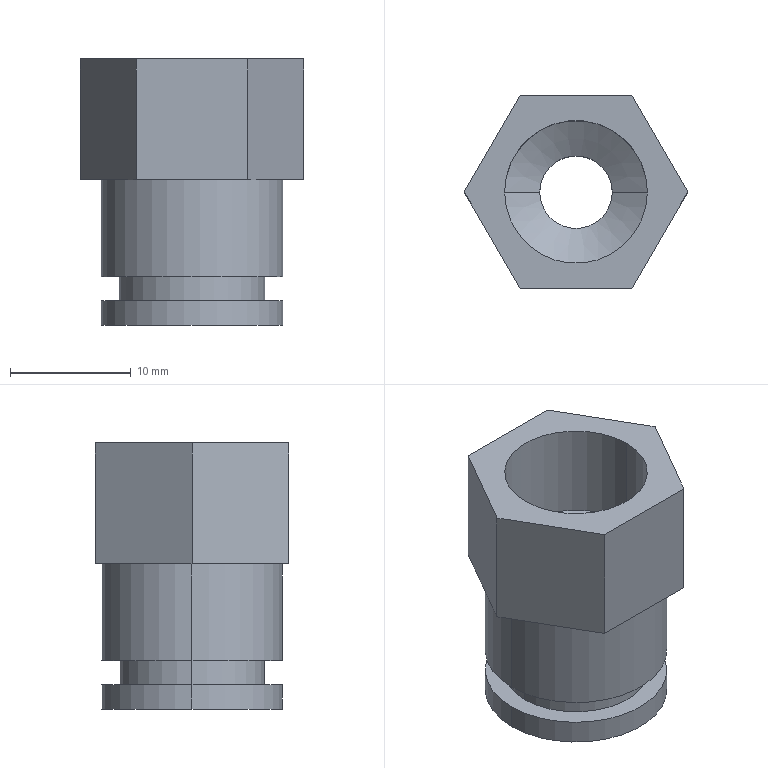Part | SolidWorks | features ICE 4, Extrusion 1, HoleWzd 1 | 1 solid | 23 faces | box 18.475 x 16 x 22 mm | volume 2877 mm3 | plane 11 | cylinder 10 | cone 2 | commonest cylinder face diameters 15 x4 6 x2 11.8 x2 12 x2
STEP:
#1=CARTESIAN_POINT('',(-5.9,0.,14.));
#2=VERTEX_POINT('',#1);
#3=CARTESIAN_POINT('',(5.9,0.,14.));
#4=VERTEX_POINT('',#3);
#5=CARTESIAN_POINT('',(0.,0.,14.));
#6=DIRECTION('',(0.,0.,1.));
#7=DIRECTION('',(1.,0.,0.));
#8=AXIS2_PLACEMENT_3D('',#5,#6,#7);
#9=CIRCLE('',#8,5.9);
#10=EDGE_CURVE('',#2,#4,#9,.T.);
#11=ORIENTED_EDGE('',*,*,#10,.F.);
#12=CARTESIAN_POINT('',(-5.9,0.,22.));
#13=VERTEX_POINT('',#12);
#14=CARTESIAN_POINT('',(-5.9,0.,22.));
#15=DIRECTION('',(0.,0.,1.));
#16=VECTOR('',#15,1000.);
#17=LINE('',#14,#16);
#18=EDGE_CURVE('',#2,#13,#17,.T.);
#19=ORIENTED_EDGE('',*,*,#18,.T.);
#20=CARTESIAN_POINT('',(5.9,0.,22.));
#21=VERTEX_POINT('',#20);
#22=CARTESIAN_POINT('',(0.,0.,22.));
#23=DIRECTION('',(0.,0.,1.));
#24=DIRECTION('',(1.,0.,0.));
#25=AXIS2_PLACEMENT_3D('',#22,#23,#24);
#26=CIRCLE('',#25,5.9);
#27=EDGE_CURVE('',#13,#21,#26,.T.);
#28=ORIENTED_EDGE('',*,*,#27,.T.);
#29=CARTESIAN_POINT('',(5.9,0.,22.));
#30=DIRECTION('',(0.,0.,1.));
#31=VECTOR('',#30,1000.);
#32=LINE('',#29,#31);
#33=EDGE_CURVE('',#4,#21,#32,.T.);
#34=ORIENTED_EDGE('',*,*,#33,.F.);
#35=EDGE_LOOP('',(#11,#19,#28,#34));
#36=FACE_OUTER_BOUND('',#35,.T.);
#37=CARTESIAN_POINT('',(0.,0.,22.));
#38=DIRECTION('',(0.,0.,1.));
#39=DIRECTION('',(1.,0.,0.));
#40=AXIS2_PLACEMENT_3D('',#37,#38,#39);
#41=CYLINDRICAL_SURFACE('',#40,5.9);
#42=ADVANCED_FACE('',(#36),#41,.F.);
#43=CARTESIAN_POINT('',(-3.,0.,12.258));
#44=VERTEX_POINT('',#43);
#45=CARTESIAN_POINT('',(3.,0.,12.258));
#46=VERTEX_POINT('',#45);
#47=CARTESIAN_POINT('',(0.,0.,12.258));
#48=DIRECTION('',(0.,0.,1.));
#49=DIRECTION('',(1.,0.,0.));
#50=AXIS2_PLACEMENT_3D('',#47,#48,#49);
#51=CIRCLE('',#50,3.);
#52=EDGE_CURVE('',#44,#46,#51,.T.);
#53=ORIENTED_EDGE('',*,*,#52,.F.);
#54=CARTESIAN_POINT('',(-5.9,0.,14.));
#55=DIRECTION('',(-0.8572,0.,0.515));
#56=VECTOR('',#55,1000.);
#57=LINE('',#54,#56);
#58=EDGE_CURVE('',#44,#2,#57,.T.);
#59=ORIENTED_EDGE('',*,*,#58,.T.);
#60=ORIENTED_EDGE('',*,*,#10,.T.);
#61=CARTESIAN_POINT('',(5.9,0.,14.));
#62=DIRECTION('',(0.8572,0.,0.515));
#63=VECTOR('',#62,1000.);
#64=LINE('',#61,#63);
#65=EDGE_CURVE('',#46,#4,#64,.T.);
#66=ORIENTED_EDGE('',*,*,#65,.F.);
#67=EDGE_LOOP('',(#53,#59,#60,#66));
#68=FACE_OUTER_BOUND('',#67,.T.);
#69=CARTESIAN_POINT('',(0.,0.,14.));
#70=DIRECTION('',(0.,0.,1.));
#71=DIRECTION('',(1.,0.,0.));
#72=AXIS2_PLACEMENT_3D('',#69,#70,#71);
#73=CONICAL_SURFACE('',#72,5.9,1.03);
#74=ADVANCED_FACE('',(#68),#73,.F.);
#75=ORIENTED_EDGE('',*,*,#52,.T.);
#76=CARTESIAN_POINT('',(3.,0.,0.));
#77=VERTEX_POINT('',#76);
#78=CARTESIAN_POINT('',(3.,0.,22.));
#79=DIRECTION('',(0.,0.,-1.));
#80=VECTOR('',#79,1000.);
#81=LINE('',#78,#80);
#82=EDGE_CURVE('',#46,#77,#81,.T.);
#83=ORIENTED_EDGE('',*,*,#82,.T.);
#84=CARTESIAN_POINT('',(-3.,0.,0.));
#85=VERTEX_POINT('',#84);
#86=CARTESIAN_POINT('',(0.,0.,0.));
#87=DIRECTION('',(0.,0.,-1.));
#88=DIRECTION('',(-1.,0.,0.));
#89=AXIS2_PLACEMENT_3D('',#86,#87,#88);
#90=CIRCLE('',#89,3.);
#91=EDGE_CURVE('',#77,#85,#90,.T.);
#92=ORIENTED_EDGE('',*,*,#91,.T.);
#93=CARTESIAN_POINT('',(-3.,0.,22.));
#94=DIRECTION('',(0.,0.,-1.));
#95=VECTOR('',#94,1000.);
#96=LINE('',#93,#95);
#97=EDGE_CURVE('',#44,#85,#96,.T.);
#98=ORIENTED_EDGE('',*,*,#97,.F.);
#99=EDGE_LOOP('',(#75,#83,#92,#98));
#100=FACE_OUTER_BOUND('',#99,.T.);
#101=CARTESIAN_POINT('',(0.,0.,22.));
#102=DIRECTION('',(0.,0.,-1.));
#103=DIRECTION('',(-1.,0.,0.));
#104=AXIS2_PLACEMENT_3D('',#101,#102,#103);
#105=CYLINDRICAL_SURFACE('',#104,3.);
#106=ADVANCED_FACE('',(#100),#105,.F.);
#107=CARTESIAN_POINT('',(7.5,0.,12.));
#108=VERTEX_POINT('',#107);
#109=CARTESIAN_POINT('',(-7.5,0.,12.));
#110=VERTEX_POINT('',#109);
#111=CARTESIAN_POINT('',(0.,0.,12.));
#112=DIRECTION('',(0.,0.,1.));
#113=DIRECTION('',(1.,0.,0.));
#114=AXIS2_PLACEMENT_3D('',#111,#112,#113);
#115=CIRCLE('',#114,7.5);
#116=EDGE_CURVE('',#108,#110,#115,.T.);
#117=ORIENTED_EDGE('',*,*,#116,.F.);
#118=CARTESIAN_POINT('',(7.5,0.,4.));
#119=VERTEX_POINT('',#118);
#120=CARTESIAN_POINT('',(7.5,0.,12.));
#121=DIRECTION('',(0.,0.,-1.));
#122=VECTOR('',#121,1000.);
#123=LINE('',#120,#122);
#124=EDGE_CURVE('',#108,#119,#123,.T.);
#125=ORIENTED_EDGE('',*,*,#124,.T.);
#126=CARTESIAN_POINT('',(-7.5,0.,4.));
#127=VERTEX_POINT('',#126);
#128=CARTESIAN_POINT('',(0.,0.,4.));
#129=DIRECTION('',(0.,0.,1.));
#130=DIRECTION('',(1.,0.,0.));
#131=AXIS2_PLACEMENT_3D('',#128,#129,#130);
#132=CIRCLE('',#131,7.5);
#133=EDGE_CURVE('',#119,#127,#132,.T.);
#134=ORIENTED_EDGE('',*,*,#133,.T.);
#135=CARTESIAN_POINT('',(-7.5,0.,12.));
#136=DIRECTION('',(0.,0.,-1.));
#137=VECTOR('',#136,1000.);
#138=LINE('',#135,#137);
#139=EDGE_CURVE('',#110,#127,#138,.T.);
#140=ORIENTED_EDGE('',*,*,#139,.F.);
#141=EDGE_LOOP('',(#117,#125,#134,#140));
#142=FACE_OUTER_BOUND('',#141,.T.);
#143=CARTESIAN_POINT('',(0.,0.,12.));
#144=DIRECTION('',(0.,0.,-1.));
#145=DIRECTION('',(-1.,0.,0.));
#146=AXIS2_PLACEMENT_3D('',#143,#144,#145);
#147=CYLINDRICAL_SURFACE('',#146,7.5);
#148=ADVANCED_FACE('',(#142),#147,.T.);
#149=CARTESIAN_POINT('',(6.,0.,4.));
#150=VERTEX_POINT('',#149);
#151=CARTESIAN_POINT('',(-6.,0.,4.));
#152=VERTEX_POINT('',#151);
#153=CARTESIAN_POINT('',(0.,0.,4.));
#154=DIRECTION('',(0.,0.,1.));
#155=DIRECTION('',(1.,0.,0.));
#156=AXIS2_PLACEMENT_3D('',#153,#154,#155);
#157=CIRCLE('',#156,6.);
#158=EDGE_CURVE('',#150,#152,#157,.T.);
#159=ORIENTED_EDGE('',*,*,#158,.F.);
#160=CARTESIAN_POINT('',(6.,0.,2.));
#161=VERTEX_POINT('',#160);
#162=CARTESIAN_POINT('',(6.,0.,4.));
#163=DIRECTION('',(0.,0.,-1.));
#164=VECTOR('',#163,1000.);
#165=LINE('',#162,#164);
#166=EDGE_CURVE('',#150,#161,#165,.T.);
#167=ORIENTED_EDGE('',*,*,#166,.T.);
#168=CARTESIAN_POINT('',(-6.,0.,2.));
#169=VERTEX_POINT('',#168);
#170=CARTESIAN_POINT('',(0.,0.,2.));
#171=DIRECTION('',(0.,0.,1.));
#172=DIRECTION('',(1.,0.,0.));
#173=AXIS2_PLACEMENT_3D('',#170,#171,#172);
#174=CIRCLE('',#173,6.);
#175=EDGE_CURVE('',#161,#169,#174,.T.);
#176=ORIENTED_EDGE('',*,*,#175,.T.);
#177=CARTESIAN_POINT('',(-6.,0.,4.));
#178=DIRECTION('',(0.,0.,-1.));
#179=VECTOR('',#178,1000.);
#180=LINE('',#177,#179);
#181=EDGE_CURVE('',#152,#169,#180,.T.);
#182=ORIENTED_EDGE('',*,*,#181,.F.);
#183=EDGE_LOOP('',(#159,#167,#176,#182));
#184=FACE_OUTER_BOUND('',#183,.T.);
#185=CARTESIAN_POINT('',(0.,0.,4.));
#186=DIRECTION('',(0.,0.,-1.));
#187=DIRECTION('',(-1.,0.,0.));
#188=AXIS2_PLACEMENT_3D('',#185,#186,#187);
#189=CYLINDRICAL_SURFACE('',#188,6.);
#190=ADVANCED_FACE('',(#184),#189,.T.);
#191=CARTESIAN_POINT('',(7.5,0.,2.));
#192=VERTEX_POINT('',#191);
#193=CARTESIAN_POINT('',(-7.5,0.,2.));
#194=VERTEX_POINT('',#193);
#195=CARTESIAN_POINT('',(0.,0.,2.));
#196=DIRECTION('',(0.,0.,1.));
#197=DIRECTION('',(1.,0.,0.));
#198=AXIS2_PLACEMENT_3D('',#195,#196,#197);
#199=CIRCLE('',#198,7.5);
#200=EDGE_CURVE('',#192,#194,#199,.T.);
#201=ORIENTED_EDGE('',*,*,#200,.F.);
#202=CARTESIAN_POINT('',(7.5,0.,0.));
#203=VERTEX_POINT('',#202);
#204=CARTESIAN_POINT('',(7.5,0.,2.));
#205=DIRECTION('',(0.,0.,-1.));
#206=VECTOR('',#205,1000.);
#207=LINE('',#204,#206);
#208=EDGE_CURVE('',#192,#203,#207,.T.);
#209=ORIENTED_EDGE('',*,*,#208,.T.);
#210=CARTESIAN_POINT('',(-7.5,0.,0.));
#211=VERTEX_POINT('',#210);
#212=CARTESIAN_POINT('',(0.,0.,0.));
#213=DIRECTION('',(0.,0.,1.));
#214=DIRECTION('',(1.,0.,0.));
#215=AXIS2_PLACEMENT_3D('',#212,#213,#214);
#216=CIRCLE('',#215,7.5);
#217=EDGE_CURVE('',#203,#211,#216,.T.);
#218=ORIENTED_EDGE('',*,*,#217,.T.);
#219=CARTESIAN_POINT('',(-7.5,0.,2.));
#220=DIRECTION('',(0.,0.,-1.));
#221=VECTOR('',#220,1000.);
#222=LINE('',#219,#221);
#223=EDGE_CURVE('',#194,#211,#222,.T.);
#224=ORIENTED_EDGE('',*,*,#223,.F.);
#225=EDGE_LOOP('',(#201,#209,#218,#224));
#226=FACE_OUTER_BOUND('',#225,.T.);
#227=CARTESIAN_POINT('',(0.,0.,2.));
#228=DIRECTION('',(0.,0.,-1.));
#229=DIRECTION('',(-1.,0.,0.));
#230=AXIS2_PLACEMENT_3D('',#227,#228,#229);
#231=CYLINDRICAL_SURFACE('',#230,7.5);
#232=ADVANCED_FACE('',(#226),#231,.T.);
#233=ORIENTED_EDGE('',*,*,#208,.F.);
#234=CARTESIAN_POINT('',(0.,0.,2.));
#235=DIRECTION('',(0.,0.,1.));
#236=DIRECTION('',(1.,0.,0.));
#237=AXIS2_PLACEMENT_3D('',#234,#235,#236);
#238=CIRCLE('',#237,7.5);
#239=EDGE_CURVE('',#194,#192,#238,.T.);
#240=ORIENTED_EDGE('',*,*,#239,.F.);
#241=ORIENTED_EDGE('',*,*,#223,.T.);
#242=CARTESIAN_POINT('',(0.,0.,0.));
#243=DIRECTION('',(0.,0.,1.));
#244=DIRECTION('',(1.,0.,0.));
#245=AXIS2_PLACEMENT_3D('',#242,#243,#244);
#246=CIRCLE('',#245,7.5);
#247=EDGE_CURVE('',#211,#203,#246,.T.);
#248=ORIENTED_EDGE('',*,*,#247,.T.);
#249=EDGE_LOOP('',(#233,#240,#241,#248));
#250=FACE_OUTER_BOUND('',#249,.T.);
#251=CARTESIAN_POINT('',(0.,0.,2.));
#252=DIRECTION('',(0.,0.,-1.));
#253=DIRECTION('',(-1.,0.,0.));
#254=AXIS2_PLACEMENT_3D('',#251,#252,#253);
#255=CYLINDRICAL_SURFACE('',#254,7.5);
#256=ADVANCED_FACE('',(#250),#255,.T.);
#257=CARTESIAN_POINT('',(0.,0.,2.));
#258=DIRECTION('',(0.,0.,1.));
#259=DIRECTION('',(1.,0.,0.));
#260=AXIS2_PLACEMENT_3D('',#257,#258,#259);
#261=CIRCLE('',#260,6.);
#262=EDGE_CURVE('',#169,#161,#261,.T.);
#263=ORIENTED_EDGE('',*,*,#262,.F.);
#264=ORIENTED_EDGE('',*,*,#175,.F.);
#265=EDGE_LOOP('',(#263,#264));
#266=FACE_BOUND('',#265,.T.);
#267=ORIENTED_EDGE('',*,*,#239,.T.);
#268=ORIENTED_EDGE('',*,*,#200,.T.);
#269=EDGE_LOOP('',(#267,#268));
#270=FACE_OUTER_BOUND('',#269,.T.);
#271=CARTESIAN_POINT('',(0.,0.,2.));
#272=DIRECTION('',(0.,0.,1.));
#273=DIRECTION('',(1.,0.,0.));
#274=AXIS2_PLACEMENT_3D('',#271,#272,#273);
#275=PLANE('',#274);
#276=ADVANCED_FACE('',(#266,#270),#275,.T.);
#277=CARTESIAN_POINT('',(0.,0.,0.));
#278=DIRECTION('',(0.,0.,-1.));
#279=DIRECTION('',(-1.,0.,0.));
#280=AXIS2_PLACEMENT_3D('',#277,#278,#279);
#281=CIRCLE('',#280,3.);
#282=EDGE_CURVE('',#85,#77,#281,.T.);
#283=ORIENTED_EDGE('',*,*,#282,.F.);
#284=ORIENTED_EDGE('',*,*,#91,.F.);
#285=EDGE_LOOP('',(#283,#284));
#286=FACE_BOUND('',#285,.T.);
#287=ORIENTED_EDGE('',*,*,#247,.F.);
#288=ORIENTED_EDGE('',*,*,#217,.F.);
#289=EDGE_LOOP('',(#287,#288));
#290=FACE_OUTER_BOUND('',#289,.T.);
#291=CARTESIAN_POINT('',(0.,0.,0.));
#292=DIRECTION('',(0.,0.,1.));
#293=DIRECTION('',(1.,0.,0.));
#294=AXIS2_PLACEMENT_3D('',#291,#292,#293);
#295=PLANE('',#294);
#296=ADVANCED_FACE('',(#286,#290),#295,.F.);
#297=ORIENTED_EDGE('',*,*,#166,.F.);
#298=CARTESIAN_POINT('',(0.,0.,4.));
#299=DIRECTION('',(0.,0.,1.));
#300=DIRECTION('',(1.,0.,0.));
#301=AXIS2_PLACEMENT_3D('',#298,#299,#300);
#302=CIRCLE('',#301,6.);
#303=EDGE_CURVE('',#152,#150,#302,.T.);
#304=ORIENTED_EDGE('',*,*,#303,.F.);
#305=ORIENTED_EDGE('',*,*,#181,.T.);
#306=ORIENTED_EDGE('',*,*,#262,.T.);
#307=EDGE_LOOP('',(#297,#304,#305,#306));
#308=FACE_OUTER_BOUND('',#307,.T.);
#309=CARTESIAN_POINT('',(0.,0.,4.));
#310=DIRECTION('',(0.,0.,-1.));
#311=DIRECTION('',(-1.,0.,0.));
#312=AXIS2_PLACEMENT_3D('',#309,#310,#311);
#313=CYLINDRICAL_SURFACE('',#312,6.);
#314=ADVANCED_FACE('',(#308),#313,.T.);
#315=ORIENTED_EDGE('',*,*,#124,.F.);
#316=CARTESIAN_POINT('',(0.,0.,12.));
#317=DIRECTION('',(0.,0.,1.));
#318=DIRECTION('',(1.,0.,0.));
#319=AXIS2_PLACEMENT_3D('',#316,#317,#318);
#320=CIRCLE('',#319,7.5);
#321=EDGE_CURVE('',#110,#108,#320,.T.);
#322=ORIENTED_EDGE('',*,*,#321,.F.);
#323=ORIENTED_EDGE('',*,*,#139,.T.);
#324=CARTESIAN_POINT('',(0.,0.,4.));
#325=DIRECTION('',(0.,0.,1.));
#326=DIRECTION('',(1.,0.,0.));
#327=AXIS2_PLACEMENT_3D('',#324,#325,#326);
#328=CIRCLE('',#327,7.5);
#329=EDGE_CURVE('',#127,#119,#328,.T.);
#330=ORIENTED_EDGE('',*,*,#329,.T.);
#331=EDGE_LOOP('',(#315,#322,#323,#330));
#332=FACE_OUTER_BOUND('',#331,.T.);
#333=CARTESIAN_POINT('',(0.,0.,12.));
#334=DIRECTION('',(0.,0.,-1.));
#335=DIRECTION('',(-1.,0.,0.));
#336=AXIS2_PLACEMENT_3D('',#333,#334,#335);
#337=CYLINDRICAL_SURFACE('',#336,7.5);
#338=ADVANCED_FACE('',(#332),#337,.T.);
#339=ORIENTED_EDGE('',*,*,#303,.T.);
#340=ORIENTED_EDGE('',*,*,#158,.T.);
#341=EDGE_LOOP('',(#339,#340));
#342=FACE_BOUND('',#341,.T.);
#343=ORIENTED_EDGE('',*,*,#329,.F.);
#344=ORIENTED_EDGE('',*,*,#133,.F.);
#345=EDGE_LOOP('',(#343,#344));
#346=FACE_OUTER_BOUND('',#345,.T.);
#347=CARTESIAN_POINT('',(0.,0.,4.));
#348=DIRECTION('',(0.,0.,1.));
#349=DIRECTION('',(1.,0.,0.));
#350=AXIS2_PLACEMENT_3D('',#347,#348,#349);
#351=PLANE('',#350);
#352=ADVANCED_FACE('',(#342,#346),#351,.F.);
#353=CARTESIAN_POINT('',(4.619,-8.,12.));
#354=VERTEX_POINT('',#353);
#355=CARTESIAN_POINT('',(9.238,0.,12.));
#356=VERTEX_POINT('',#355);
#357=CARTESIAN_POINT('',(4.619,-8.,12.));
#358=DIRECTION('',(0.5,0.866,0.));
#359=VECTOR('',#358,1000.);
#360=LINE('',#357,#359);
#361=EDGE_CURVE('',#354,#356,#360,.T.);
#362=ORIENTED_EDGE('',*,*,#361,.T.);
#363=CARTESIAN_POINT('',(9.238,0.,22.));
#364=VERTEX_POINT('',#363);
#365=CARTESIAN_POINT('',(9.238,0.,22.));
#366=DIRECTION('',(0.,0.,-1.));
#367=VECTOR('',#366,1000.);
#368=LINE('',#365,#367);
#369=EDGE_CURVE('',#364,#356,#368,.T.);
#370=ORIENTED_EDGE('',*,*,#369,.F.);
#371=CARTESIAN_POINT('',(4.619,-8.,22.));
#372=VERTEX_POINT('',#371);
#373=CARTESIAN_POINT('',(4.619,-8.,22.));
#374=DIRECTION('',(0.5,0.866,0.));
#375=VECTOR('',#374,1000.);
#376=LINE('',#373,#375);
#377=EDGE_CURVE('',#372,#364,#376,.T.);
#378=ORIENTED_EDGE('',*,*,#377,.F.);
#379=CARTESIAN_POINT('',(4.619,-8.,22.));
#380=DIRECTION('',(0.,0.,-1.));
#381=VECTOR('',#380,1000.);
#382=LINE('',#379,#381);
#383=EDGE_CURVE('',#372,#354,#382,.T.);
#384=ORIENTED_EDGE('',*,*,#383,.T.);
#385=EDGE_LOOP('',(#362,#370,#378,#384));
#386=FACE_OUTER_BOUND('',#385,.T.);
#387=CARTESIAN_POINT('',(4.619,-8.,22.));
#388=DIRECTION('',(-0.866,0.5,0.));
#389=DIRECTION('',(-0.5,-0.866,0.));
#390=AXIS2_PLACEMENT_3D('',#387,#388,#389);
#391=PLANE('',#390);
#392=ADVANCED_FACE('',(#386),#391,.F.);
#393=CARTESIAN_POINT('',(4.619,8.,12.));
#394=VERTEX_POINT('',#393);
#395=CARTESIAN_POINT('',(9.238,0.,12.));
#396=DIRECTION('',(-0.5,0.866,0.));
#397=VECTOR('',#396,1000.);
#398=LINE('',#395,#397);
#399=EDGE_CURVE('',#356,#394,#398,.T.);
#400=ORIENTED_EDGE('',*,*,#399,.T.);
#401=CARTESIAN_POINT('',(4.619,8.,22.));
#402=VERTEX_POINT('',#401);
#403=CARTESIAN_POINT('',(4.619,8.,22.));
#404=DIRECTION('',(0.,0.,-1.));
#405=VECTOR('',#404,1000.);
#406=LINE('',#403,#405);
#407=EDGE_CURVE('',#402,#394,#406,.T.);
#408=ORIENTED_EDGE('',*,*,#407,.F.);
#409=CARTESIAN_POINT('',(9.238,0.,22.));
#410=DIRECTION('',(-0.5,0.866,0.));
#411=VECTOR('',#410,1000.);
#412=LINE('',#409,#411);
#413=EDGE_CURVE('',#364,#402,#412,.T.);
#414=ORIENTED_EDGE('',*,*,#413,.F.);
#415=ORIENTED_EDGE('',*,*,#369,.T.);
#416=EDGE_LOOP('',(#400,#408,#414,#415));
#417=FACE_OUTER_BOUND('',#416,.T.);
#418=CARTESIAN_POINT('',(9.238,0.,22.));
#419=DIRECTION('',(-0.866,-0.5,0.));
#420=DIRECTION('',(0.5,-0.866,0.));
#421=AXIS2_PLACEMENT_3D('',#418,#419,#420);
#422=PLANE('',#421);
#423=ADVANCED_FACE('',(#417),#422,.F.);
#424=CARTESIAN_POINT('',(-4.619,8.,12.));
#425=VERTEX_POINT('',#424);
#426=CARTESIAN_POINT('',(4.619,8.,12.));
#427=DIRECTION('',(-1.,0.,0.));
#428=VECTOR('',#427,1000.);
#429=LINE('',#426,#428);
#430=EDGE_CURVE('',#394,#425,#429,.T.);
#431=ORIENTED_EDGE('',*,*,#430,.T.);
#432=CARTESIAN_POINT('',(-4.619,8.,22.));
#433=VERTEX_POINT('',#432);
#434=CARTESIAN_POINT('',(-4.619,8.,22.));
#435=DIRECTION('',(0.,0.,-1.));
#436=VECTOR('',#435,1000.);
#437=LINE('',#434,#436);
#438=EDGE_CURVE('',#433,#425,#437,.T.);
#439=ORIENTED_EDGE('',*,*,#438,.F.);
#440=CARTESIAN_POINT('',(4.619,8.,22.));
#441=DIRECTION('',(-1.,0.,0.));
#442=VECTOR('',#441,1000.);
#443=LINE('',#440,#442);
#444=EDGE_CURVE('',#402,#433,#443,.T.);
#445=ORIENTED_EDGE('',*,*,#444,.F.);
#446=ORIENTED_EDGE('',*,*,#407,.T.);
#447=EDGE_LOOP('',(#431,#439,#445,#446));
#448=FACE_OUTER_BOUND('',#447,.T.);
#449=CARTESIAN_POINT('',(4.619,8.,22.));
#450=DIRECTION('',(0.,-1.,0.));
#451=DIRECTION('',(1.,0.,0.));
#452=AXIS2_PLACEMENT_3D('',#449,#450,#451);
#453=PLANE('',#452);
#454=ADVANCED_FACE('',(#448),#453,.F.);
#455=CARTESIAN_POINT('',(-9.238,0.,12.));
#456=VERTEX_POINT('',#455);
#457=CARTESIAN_POINT('',(-4.619,8.,12.));
#458=DIRECTION('',(-0.5,-0.866,0.));
#459=VECTOR('',#458,1000.);
#460=LINE('',#457,#459);
#461=EDGE_CURVE('',#425,#456,#460,.T.);
#462=ORIENTED_EDGE('',*,*,#461,.T.);
#463=CARTESIAN_POINT('',(-9.238,0.,22.));
#464=VERTEX_POINT('',#463);
#465=CARTESIAN_POINT('',(-9.238,0.,22.));
#466=DIRECTION('',(0.,0.,-1.));
#467=VECTOR('',#466,1000.);
#468=LINE('',#465,#467);
#469=EDGE_CURVE('',#464,#456,#468,.T.);
#470=ORIENTED_EDGE('',*,*,#469,.F.);
#471=CARTESIAN_POINT('',(-4.619,8.,22.));
#472=DIRECTION('',(-0.5,-0.866,0.));
#473=VECTOR('',#472,1000.);
#474=LINE('',#471,#473);
#475=EDGE_CURVE('',#433,#464,#474,.T.);
#476=ORIENTED_EDGE('',*,*,#475,.F.);
#477=ORIENTED_EDGE('',*,*,#438,.T.);
#478=EDGE_LOOP('',(#462,#470,#476,#477));
#479=FACE_OUTER_BOUND('',#478,.T.);
#480=CARTESIAN_POINT('',(-4.619,8.,22.));
#481=DIRECTION('',(0.866,-0.5,0.));
#482=DIRECTION('',(0.5,0.866,0.));
#483=AXIS2_PLACEMENT_3D('',#480,#481,#482);
#484=PLANE('',#483);
#485=ADVANCED_FACE('',(#479),#484,.F.);
#486=CARTESIAN_POINT('',(-4.619,-8.,12.));
#487=VERTEX_POINT('',#486);
#488=CARTESIAN_POINT('',(-9.238,0.,12.));
#489=DIRECTION('',(0.5,-0.866,0.));
#490=VECTOR('',#489,1000.);
#491=LINE('',#488,#490);
#492=EDGE_CURVE('',#456,#487,#491,.T.);
#493=ORIENTED_EDGE('',*,*,#492,.T.);
#494=CARTESIAN_POINT('',(-4.619,-8.,22.));
#495=VERTEX_POINT('',#494);
#496=CARTESIAN_POINT('',(-4.619,-8.,22.));
#497=DIRECTION('',(0.,0.,-1.));
#498=VECTOR('',#497,1000.);
#499=LINE('',#496,#498);
#500=EDGE_CURVE('',#495,#487,#499,.T.);
#501=ORIENTED_EDGE('',*,*,#500,.F.);
#502=CARTESIAN_POINT('',(-9.238,0.,22.));
#503=DIRECTION('',(0.5,-0.866,0.));
#504=VECTOR('',#503,1000.);
#505=LINE('',#502,#504);
#506=EDGE_CURVE('',#464,#495,#505,.T.);
#507=ORIENTED_EDGE('',*,*,#506,.F.);
#508=ORIENTED_EDGE('',*,*,#469,.T.);
#509=EDGE_LOOP('',(#493,#501,#507,#508));
#510=FACE_OUTER_BOUND('',#509,.T.);
#511=CARTESIAN_POINT('',(-9.238,0.,22.));
#512=DIRECTION('',(0.866,0.5,0.));
#513=DIRECTION('',(-0.5,0.866,0.));
#514=AXIS2_PLACEMENT_3D('',#511,#512,#513);
#515=PLANE('',#514);
#516=ADVANCED_FACE('',(#510),#515,.F.);
#517=CARTESIAN_POINT('',(-4.619,-8.,12.));
#518=DIRECTION('',(1.,0.,0.));
#519=VECTOR('',#518,1000.);
#520=LINE('',#517,#519);
#521=EDGE_CURVE('',#487,#354,#520,.T.);
#522=ORIENTED_EDGE('',*,*,#521,.T.);
#523=ORIENTED_EDGE('',*,*,#383,.F.);
#524=CARTESIAN_POINT('',(-4.619,-8.,22.));
#525=DIRECTION('',(1.,0.,0.));
#526=VECTOR('',#525,1000.);
#527=LINE('',#524,#526);
#528=EDGE_CURVE('',#495,#372,#527,.T.);
#529=ORIENTED_EDGE('',*,*,#528,.F.);
#530=ORIENTED_EDGE('',*,*,#500,.T.);
#531=EDGE_LOOP('',(#522,#523,#529,#530));
#532=FACE_OUTER_BOUND('',#531,.T.);
#533=CARTESIAN_POINT('',(-4.619,-8.,22.));
#534=DIRECTION('',(0.,1.,0.));
#535=DIRECTION('',(-1.,0.,0.));
#536=AXIS2_PLACEMENT_3D('',#533,#534,#535);
#537=PLANE('',#536);
#538=ADVANCED_FACE('',(#532),#537,.F.);
#539=CARTESIAN_POINT('',(0.,0.,22.));
#540=DIRECTION('',(0.,0.,1.));
#541=DIRECTION('',(1.,0.,0.));
#542=AXIS2_PLACEMENT_3D('',#539,#540,#541);
#543=CIRCLE('',#542,5.9);
#544=EDGE_CURVE('',#21,#13,#543,.T.);
#545=ORIENTED_EDGE('',*,*,#544,.F.);
#546=ORIENTED_EDGE('',*,*,#27,.F.);
#547=EDGE_LOOP('',(#545,#546));
#548=FACE_BOUND('',#547,.T.);
#549=ORIENTED_EDGE('',*,*,#377,.T.);
#550=ORIENTED_EDGE('',*,*,#413,.T.);
#551=ORIENTED_EDGE('',*,*,#444,.T.);
#552=ORIENTED_EDGE('',*,*,#475,.T.);
#553=ORIENTED_EDGE('',*,*,#506,.T.);
#554=ORIENTED_EDGE('',*,*,#528,.T.);
#555=EDGE_LOOP('',(#549,#550,#551,#552,#553,#554));
#556=FACE_OUTER_BOUND('',#555,.T.);
#557=CARTESIAN_POINT('',(0.,0.,22.));
#558=DIRECTION('',(0.,0.,1.));
#559=DIRECTION('',(1.,0.,0.));
#560=AXIS2_PLACEMENT_3D('',#557,#558,#559);
#561=PLANE('',#560);
#562=ADVANCED_FACE('',(#548,#556),#561,.T.);
#563=ORIENTED_EDGE('',*,*,#321,.T.);
#564=ORIENTED_EDGE('',*,*,#116,.T.);
#565=EDGE_LOOP('',(#563,#564));
#566=FACE_BOUND('',#565,.T.);
#567=ORIENTED_EDGE('',*,*,#361,.F.);
#568=ORIENTED_EDGE('',*,*,#521,.F.);
#569=ORIENTED_EDGE('',*,*,#492,.F.);
#570=ORIENTED_EDGE('',*,*,#461,.F.);
#571=ORIENTED_EDGE('',*,*,#430,.F.);
#572=ORIENTED_EDGE('',*,*,#399,.F.);
#573=EDGE_LOOP('',(#567,#568,#569,#570,#571,#572));
#574=FACE_OUTER_BOUND('',#573,.T.);
#575=CARTESIAN_POINT('',(0.,0.,12.));
#576=DIRECTION('',(0.,0.,1.));
#577=DIRECTION('',(1.,0.,0.));
#578=AXIS2_PLACEMENT_3D('',#575,#576,#577);
#579=PLANE('',#578);
#580=ADVANCED_FACE('',(#566,#574),#579,.F.);
#581=ORIENTED_EDGE('',*,*,#82,.F.);
#582=CARTESIAN_POINT('',(0.,0.,12.258));
#583=DIRECTION('',(0.,0.,1.));
#584=DIRECTION('',(1.,0.,0.));
#585=AXIS2_PLACEMENT_3D('',#582,#583,#584);
#586=CIRCLE('',#585,3.);
#587=EDGE_CURVE('',#46,#44,#586,.T.);
#588=ORIENTED_EDGE('',*,*,#587,.T.);
#589=ORIENTED_EDGE('',*,*,#97,.T.);
#590=ORIENTED_EDGE('',*,*,#282,.T.);
#591=EDGE_LOOP('',(#581,#588,#589,#590));
#592=FACE_OUTER_BOUND('',#591,.T.);
#593=CARTESIAN_POINT('',(0.,0.,22.));
#594=DIRECTION('',(0.,0.,-1.));
#595=DIRECTION('',(-1.,0.,0.));
#596=AXIS2_PLACEMENT_3D('',#593,#594,#595);
#597=CYLINDRICAL_SURFACE('',#596,3.);
#598=ADVANCED_FACE('',(#592),#597,.F.);
#599=ORIENTED_EDGE('',*,*,#58,.F.);
#600=ORIENTED_EDGE('',*,*,#587,.F.);
#601=ORIENTED_EDGE('',*,*,#65,.T.);
#602=CARTESIAN_POINT('',(0.,0.,14.));
#603=DIRECTION('',(0.,0.,1.));
#604=DIRECTION('',(1.,0.,0.));
#605=AXIS2_PLACEMENT_3D('',#602,#603,#604);
#606=CIRCLE('',#605,5.9);
#607=EDGE_CURVE('',#4,#2,#606,.T.);
#608=ORIENTED_EDGE('',*,*,#607,.T.);
#609=EDGE_LOOP('',(#599,#600,#601,#608));
#610=FACE_OUTER_BOUND('',#609,.T.);
#611=CARTESIAN_POINT('',(0.,0.,14.));
#612=DIRECTION('',(0.,0.,1.));
#613=DIRECTION('',(1.,0.,0.));
#614=AXIS2_PLACEMENT_3D('',#611,#612,#613);
#615=CONICAL_SURFACE('',#614,5.9,1.03);
#616=ADVANCED_FACE('',(#610),#615,.F.);
#617=ORIENTED_EDGE('',*,*,#18,.F.);
#618=ORIENTED_EDGE('',*,*,#607,.F.);
#619=ORIENTED_EDGE('',*,*,#33,.T.);
#620=ORIENTED_EDGE('',*,*,#544,.T.);
#621=EDGE_LOOP('',(#617,#618,#619,#620));
#622=FACE_OUTER_BOUND('',#621,.T.);
#623=CARTESIAN_POINT('',(0.,0.,22.));
#624=DIRECTION('',(0.,0.,1.));
#625=DIRECTION('',(1.,0.,0.));
#626=AXIS2_PLACEMENT_3D('',#623,#624,#625);
#627=CYLINDRICAL_SURFACE('',#626,5.9);
#628=ADVANCED_FACE('',(#622),#627,.F.);
#629=CLOSED_SHELL('',(#42,#74,#106,#148,#190,#232,#256,#276,#296,#314,#338,#352,#392,#423,#454,#485,#516,#538,#562,#580,#598,#616,#628));
#630=MANIFOLD_SOLID_BREP('',#629);
#631=CARTESIAN_POINT('',(0.,0.,0.));
#632=DIRECTION('',(0.,0.,1.));
#633=DIRECTION('',(1.,0.,0.));
#634=AXIS2_PLACEMENT_3D('',#631,#632,#633);
#635=(LENGTH_UNIT()NAMED_UNIT(*)SI_UNIT(.MILLI.,.METRE.));
#636=UNCERTAINTY_MEASURE_WITH_UNIT(LENGTH_MEASURE(0.00001),#635,'','');
#637=(NAMED_UNIT(*)PLANE_ANGLE_UNIT()SI_UNIT($,.RADIAN.));
#638=(NAMED_UNIT(*)SI_UNIT($,.STERADIAN.)SOLID_ANGLE_UNIT());
#639=(GEOMETRIC_REPRESENTATION_CONTEXT(3)GLOBAL_UNCERTAINTY_ASSIGNED_CONTEXT((#636))GLOBAL_UNIT_ASSIGNED_CONTEXT((#635,#637,#638))REPRESENTATION_CONTEXT('',''));
#640=ADVANCED_BREP_SHAPE_REPRESENTATION('',(#630,#634),#639);